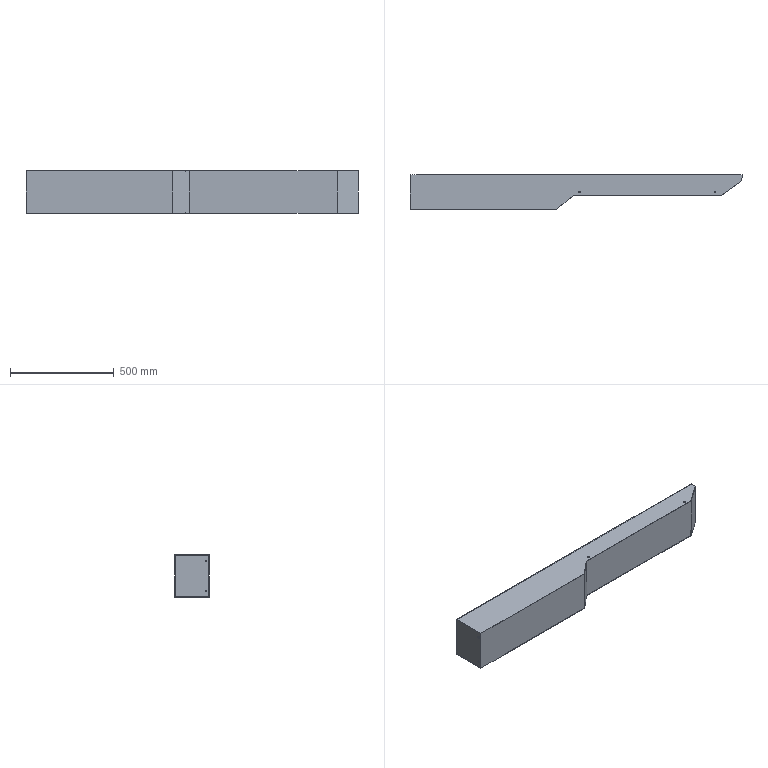Part | SolidWorks | features ICE 5, Extrusion 1, Shell 1 | 1 solid | 40 faces | box 1600 x 167 x 205 mm | volume 1759661 mm3 | plane 22 | cylinder 18 | commonest cylinder face diameters 9 x18
STEP:
#1=CARTESIAN_POINT('',(1474.53,-84.,-2.));
#2=VERTEX_POINT('',#1);
#3=CARTESIAN_POINT('',(1465.53,-84.,-2.));
#4=VERTEX_POINT('',#3);
#5=CARTESIAN_POINT('',(1470.03,-84.,-2.));
#6=DIRECTION('',(0.,0.,-1.));
#7=DIRECTION('',(-1.,0.,0.));
#8=AXIS2_PLACEMENT_3D('',#5,#6,#7);
#9=CIRCLE('',#8,4.5);
#10=EDGE_CURVE('',#2,#4,#9,.T.);
#11=ORIENTED_EDGE('',*,*,#10,.T.);
#12=CARTESIAN_POINT('',(1465.53,-84.,0.));
#13=VERTEX_POINT('',#12);
#14=CARTESIAN_POINT('',(1465.53,-84.,-110.));
#15=DIRECTION('',(0.,0.,1.));
#16=VECTOR('',#15,1000.);
#17=LINE('',#14,#16);
#18=EDGE_CURVE('',#4,#13,#17,.T.);
#19=ORIENTED_EDGE('',*,*,#18,.T.);
#20=CARTESIAN_POINT('',(1474.53,-84.,0.));
#21=VERTEX_POINT('',#20);
#22=CARTESIAN_POINT('',(1470.03,-84.,0.));
#23=DIRECTION('',(0.,0.,1.));
#24=DIRECTION('',(1.,0.,0.));
#25=AXIS2_PLACEMENT_3D('',#22,#23,#24);
#26=CIRCLE('',#25,4.5);
#27=EDGE_CURVE('',#13,#21,#26,.T.);
#28=ORIENTED_EDGE('',*,*,#27,.T.);
#29=CARTESIAN_POINT('',(1474.53,-84.,-110.));
#30=DIRECTION('',(0.,0.,1.));
#31=VECTOR('',#30,1000.);
#32=LINE('',#29,#31);
#33=EDGE_CURVE('',#2,#21,#32,.T.);
#34=ORIENTED_EDGE('',*,*,#33,.F.);
#35=EDGE_LOOP('',(#11,#19,#28,#34));
#36=FACE_OUTER_BOUND('',#35,.T.);
#37=CARTESIAN_POINT('',(1470.03,-84.,-110.));
#38=DIRECTION('',(0.,0.,1.));
#39=DIRECTION('',(1.,0.,0.));
#40=AXIS2_PLACEMENT_3D('',#37,#38,#39);
#41=CYLINDRICAL_SURFACE('',#40,4.5);
#42=ADVANCED_FACE('',(#36),#41,.F.);
#43=CARTESIAN_POINT('',(821.5,-84.,-2.));
#44=VERTEX_POINT('',#43);
#45=CARTESIAN_POINT('',(812.5,-84.,-2.));
#46=VERTEX_POINT('',#45);
#47=CARTESIAN_POINT('',(817.,-84.,-2.));
#48=DIRECTION('',(0.,0.,-1.));
#49=DIRECTION('',(-1.,0.,0.));
#50=AXIS2_PLACEMENT_3D('',#47,#48,#49);
#51=CIRCLE('',#50,4.5);
#52=EDGE_CURVE('',#44,#46,#51,.T.);
#53=ORIENTED_EDGE('',*,*,#52,.T.);
#54=CARTESIAN_POINT('',(812.5,-84.,0.));
#55=VERTEX_POINT('',#54);
#56=CARTESIAN_POINT('',(812.5,-84.,-110.));
#57=DIRECTION('',(0.,0.,1.));
#58=VECTOR('',#57,1000.);
#59=LINE('',#56,#58);
#60=EDGE_CURVE('',#46,#55,#59,.T.);
#61=ORIENTED_EDGE('',*,*,#60,.T.);
#62=CARTESIAN_POINT('',(821.5,-84.,0.));
#63=VERTEX_POINT('',#62);
#64=CARTESIAN_POINT('',(817.,-84.,0.));
#65=DIRECTION('',(0.,0.,1.));
#66=DIRECTION('',(1.,0.,0.));
#67=AXIS2_PLACEMENT_3D('',#64,#65,#66);
#68=CIRCLE('',#67,4.5);
#69=EDGE_CURVE('',#55,#63,#68,.T.);
#70=ORIENTED_EDGE('',*,*,#69,.T.);
#71=CARTESIAN_POINT('',(821.5,-84.,-110.));
#72=DIRECTION('',(0.,0.,1.));
#73=VECTOR('',#72,1000.);
#74=LINE('',#71,#73);
#75=EDGE_CURVE('',#44,#63,#74,.T.);
#76=ORIENTED_EDGE('',*,*,#75,.F.);
#77=EDGE_LOOP('',(#53,#61,#70,#76));
#78=FACE_OUTER_BOUND('',#77,.T.);
#79=CARTESIAN_POINT('',(817.,-84.,-110.));
#80=DIRECTION('',(0.,0.,1.));
#81=DIRECTION('',(1.,0.,0.));
#82=AXIS2_PLACEMENT_3D('',#79,#80,#81);
#83=CYLINDRICAL_SURFACE('',#82,4.5);
#84=ADVANCED_FACE('',(#78),#83,.F.);
#85=CARTESIAN_POINT('',(1588.5,-2.,-30.));
#86=VERTEX_POINT('',#85);
#87=CARTESIAN_POINT('',(1579.5,-2.,-30.));
#88=VERTEX_POINT('',#87);
#89=CARTESIAN_POINT('',(1584.,-2.,-30.));
#90=DIRECTION('',(0.,1.,0.));
#91=DIRECTION('',(-1.,0.,0.));
#92=AXIS2_PLACEMENT_3D('',#89,#90,#91);
#93=CIRCLE('',#92,4.5);
#94=EDGE_CURVE('',#86,#88,#93,.T.);
#95=ORIENTED_EDGE('',*,*,#94,.F.);
#96=CARTESIAN_POINT('',(1588.5,0.,-30.));
#97=VERTEX_POINT('',#96);
#98=CARTESIAN_POINT('',(1588.5,-16.,-30.));
#99=DIRECTION('',(0.,1.,0.));
#100=VECTOR('',#99,1000.);
#101=LINE('',#98,#100);
#102=EDGE_CURVE('',#86,#97,#101,.T.);
#103=ORIENTED_EDGE('',*,*,#102,.T.);
#104=CARTESIAN_POINT('',(1579.5,0.,-30.));
#105=VERTEX_POINT('',#104);
#106=CARTESIAN_POINT('',(1584.,0.,-30.));
#107=DIRECTION('',(0.,1.,0.));
#108=DIRECTION('',(-1.,0.,0.));
#109=AXIS2_PLACEMENT_3D('',#106,#107,#108);
#110=CIRCLE('',#109,4.5);
#111=EDGE_CURVE('',#97,#105,#110,.T.);
#112=ORIENTED_EDGE('',*,*,#111,.T.);
#113=CARTESIAN_POINT('',(1579.5,-16.,-30.));
#114=DIRECTION('',(0.,1.,0.));
#115=VECTOR('',#114,1000.);
#116=LINE('',#113,#115);
#117=EDGE_CURVE('',#88,#105,#116,.T.);
#118=ORIENTED_EDGE('',*,*,#117,.F.);
#119=EDGE_LOOP('',(#95,#103,#112,#118));
#120=FACE_OUTER_BOUND('',#119,.T.);
#121=CARTESIAN_POINT('',(1584.,-16.,-30.));
#122=DIRECTION('',(0.,1.,0.));
#123=DIRECTION('',(-1.,0.,0.));
#124=AXIS2_PLACEMENT_3D('',#121,#122,#123);
#125=CYLINDRICAL_SURFACE('',#124,4.5);
#126=ADVANCED_FACE('',(#120),#125,.F.);
#127=CARTESIAN_POINT('',(1588.5,-2.,-175.));
#128=VERTEX_POINT('',#127);
#129=CARTESIAN_POINT('',(1579.5,-2.,-175.));
#130=VERTEX_POINT('',#129);
#131=CARTESIAN_POINT('',(1584.,-2.,-175.));
#132=DIRECTION('',(0.,1.,0.));
#133=DIRECTION('',(-1.,0.,0.));
#134=AXIS2_PLACEMENT_3D('',#131,#132,#133);
#135=CIRCLE('',#134,4.5);
#136=EDGE_CURVE('',#128,#130,#135,.T.);
#137=ORIENTED_EDGE('',*,*,#136,.F.);
#138=CARTESIAN_POINT('',(1588.5,0.,-175.));
#139=VERTEX_POINT('',#138);
#140=CARTESIAN_POINT('',(1588.5,-16.,-175.));
#141=DIRECTION('',(0.,1.,0.));
#142=VECTOR('',#141,1000.);
#143=LINE('',#140,#142);
#144=EDGE_CURVE('',#128,#139,#143,.T.);
#145=ORIENTED_EDGE('',*,*,#144,.T.);
#146=CARTESIAN_POINT('',(1579.5,0.,-175.));
#147=VERTEX_POINT('',#146);
#148=CARTESIAN_POINT('',(1584.,0.,-175.));
#149=DIRECTION('',(0.,1.,0.));
#150=DIRECTION('',(-1.,0.,0.));
#151=AXIS2_PLACEMENT_3D('',#148,#149,#150);
#152=CIRCLE('',#151,4.5);
#153=EDGE_CURVE('',#139,#147,#152,.T.);
#154=ORIENTED_EDGE('',*,*,#153,.T.);
#155=CARTESIAN_POINT('',(1579.5,-16.,-175.));
#156=DIRECTION('',(0.,1.,0.));
#157=VECTOR('',#156,1000.);
#158=LINE('',#155,#157);
#159=EDGE_CURVE('',#130,#147,#158,.T.);
#160=ORIENTED_EDGE('',*,*,#159,.F.);
#161=EDGE_LOOP('',(#137,#145,#154,#160));
#162=FACE_OUTER_BOUND('',#161,.T.);
#163=CARTESIAN_POINT('',(1584.,-16.,-175.));
#164=DIRECTION('',(0.,1.,0.));
#165=DIRECTION('',(-1.,0.,0.));
#166=AXIS2_PLACEMENT_3D('',#163,#164,#165);
#167=CYLINDRICAL_SURFACE('',#166,4.5);
#168=ADVANCED_FACE('',(#162),#167,.F.);
#169=CARTESIAN_POINT('',(2.,-151.,-25.5));
#170=VERTEX_POINT('',#169);
#171=CARTESIAN_POINT('',(2.,-151.,-34.5));
#172=VERTEX_POINT('',#171);
#173=CARTESIAN_POINT('',(2.,-151.,-30.));
#174=DIRECTION('',(1.,0.,0.));
#175=DIRECTION('',(0.,0.,-1.));
#176=AXIS2_PLACEMENT_3D('',#173,#174,#175);
#177=CIRCLE('',#176,4.5);
#178=EDGE_CURVE('',#170,#172,#177,.T.);
#179=ORIENTED_EDGE('',*,*,#178,.T.);
#180=CARTESIAN_POINT('',(0.,-151.,-34.5));
#181=VERTEX_POINT('',#180);
#182=CARTESIAN_POINT('',(78.,-151.,-34.5));
#183=DIRECTION('',(-1.,0.,0.));
#184=VECTOR('',#183,1000.);
#185=LINE('',#182,#184);
#186=EDGE_CURVE('',#172,#181,#185,.T.);
#187=ORIENTED_EDGE('',*,*,#186,.T.);
#188=CARTESIAN_POINT('',(0.,-151.,-25.5));
#189=VERTEX_POINT('',#188);
#190=CARTESIAN_POINT('',(0.,-151.,-30.));
#191=DIRECTION('',(-1.,0.,0.));
#192=DIRECTION('',(0.,0.,1.));
#193=AXIS2_PLACEMENT_3D('',#190,#191,#192);
#194=CIRCLE('',#193,4.5);
#195=EDGE_CURVE('',#181,#189,#194,.T.);
#196=ORIENTED_EDGE('',*,*,#195,.T.);
#197=CARTESIAN_POINT('',(78.,-151.,-25.5));
#198=DIRECTION('',(-1.,0.,0.));
#199=VECTOR('',#198,1000.);
#200=LINE('',#197,#199);
#201=EDGE_CURVE('',#170,#189,#200,.T.);
#202=ORIENTED_EDGE('',*,*,#201,.F.);
#203=EDGE_LOOP('',(#179,#187,#196,#202));
#204=FACE_OUTER_BOUND('',#203,.T.);
#205=CARTESIAN_POINT('',(78.,-151.,-30.));
#206=DIRECTION('',(-1.,0.,0.));
#207=DIRECTION('',(0.,0.,1.));
#208=AXIS2_PLACEMENT_3D('',#205,#206,#207);
#209=CYLINDRICAL_SURFACE('',#208,4.5);
#210=ADVANCED_FACE('',(#204),#209,.F.);
#211=CARTESIAN_POINT('',(2.,-151.,-170.5));
#212=VERTEX_POINT('',#211);
#213=CARTESIAN_POINT('',(2.,-151.,-179.5));
#214=VERTEX_POINT('',#213);
#215=CARTESIAN_POINT('',(2.,-151.,-175.));
#216=DIRECTION('',(1.,0.,0.));
#217=DIRECTION('',(0.,0.,-1.));
#218=AXIS2_PLACEMENT_3D('',#215,#216,#217);
#219=CIRCLE('',#218,4.5);
#220=EDGE_CURVE('',#212,#214,#219,.T.);
#221=ORIENTED_EDGE('',*,*,#220,.T.);
#222=CARTESIAN_POINT('',(0.,-151.,-179.5));
#223=VERTEX_POINT('',#222);
#224=CARTESIAN_POINT('',(78.,-151.,-179.5));
#225=DIRECTION('',(-1.,0.,0.));
#226=VECTOR('',#225,1000.);
#227=LINE('',#224,#226);
#228=EDGE_CURVE('',#214,#223,#227,.T.);
#229=ORIENTED_EDGE('',*,*,#228,.T.);
#230=CARTESIAN_POINT('',(0.,-151.,-170.5));
#231=VERTEX_POINT('',#230);
#232=CARTESIAN_POINT('',(0.,-151.,-175.));
#233=DIRECTION('',(-1.,0.,0.));
#234=DIRECTION('',(0.,0.,1.));
#235=AXIS2_PLACEMENT_3D('',#232,#233,#234);
#236=CIRCLE('',#235,4.5);
#237=EDGE_CURVE('',#223,#231,#236,.T.);
#238=ORIENTED_EDGE('',*,*,#237,.T.);
#239=CARTESIAN_POINT('',(78.,-151.,-170.5));
#240=DIRECTION('',(-1.,0.,0.));
#241=VECTOR('',#240,1000.);
#242=LINE('',#239,#241);
#243=EDGE_CURVE('',#212,#231,#242,.T.);
#244=ORIENTED_EDGE('',*,*,#243,.F.);
#245=EDGE_LOOP('',(#221,#229,#238,#244));
#246=FACE_OUTER_BOUND('',#245,.T.);
#247=CARTESIAN_POINT('',(78.,-151.,-175.));
#248=DIRECTION('',(-1.,0.,0.));
#249=DIRECTION('',(0.,0.,1.));
#250=AXIS2_PLACEMENT_3D('',#247,#248,#249);
#251=CYLINDRICAL_SURFACE('',#250,4.5);
#252=ADVANCED_FACE('',(#246),#251,.F.);
#253=CARTESIAN_POINT('',(804.5,-14.,-203.));
#254=VERTEX_POINT('',#253);
#255=CARTESIAN_POINT('',(795.5,-14.,-203.));
#256=VERTEX_POINT('',#255);
#257=CARTESIAN_POINT('',(800.,-14.,-203.));
#258=DIRECTION('',(0.,0.,-1.));
#259=DIRECTION('',(-1.,0.,0.));
#260=AXIS2_PLACEMENT_3D('',#257,#258,#259);
#261=CIRCLE('',#260,4.5);
#262=EDGE_CURVE('',#254,#256,#261,.T.);
#263=ORIENTED_EDGE('',*,*,#262,.F.);
#264=CARTESIAN_POINT('',(804.5,-14.,-205.));
#265=VERTEX_POINT('',#264);
#266=CARTESIAN_POINT('',(804.5,-14.,-203.));
#267=DIRECTION('',(0.,0.,-1.));
#268=VECTOR('',#267,1000.);
#269=LINE('',#266,#268);
#270=EDGE_CURVE('',#254,#265,#269,.T.);
#271=ORIENTED_EDGE('',*,*,#270,.T.);
#272=CARTESIAN_POINT('',(795.5,-14.,-205.));
#273=VERTEX_POINT('',#272);
#274=CARTESIAN_POINT('',(800.,-14.,-205.));
#275=DIRECTION('',(0.,0.,-1.));
#276=DIRECTION('',(-1.,0.,0.));
#277=AXIS2_PLACEMENT_3D('',#274,#275,#276);
#278=CIRCLE('',#277,4.5);
#279=EDGE_CURVE('',#265,#273,#278,.T.);
#280=ORIENTED_EDGE('',*,*,#279,.T.);
#281=CARTESIAN_POINT('',(795.5,-14.,-203.));
#282=DIRECTION('',(0.,0.,-1.));
#283=VECTOR('',#282,1000.);
#284=LINE('',#281,#283);
#285=EDGE_CURVE('',#256,#273,#284,.T.);
#286=ORIENTED_EDGE('',*,*,#285,.F.);
#287=EDGE_LOOP('',(#263,#271,#280,#286));
#288=FACE_OUTER_BOUND('',#287,.T.);
#289=CARTESIAN_POINT('',(800.,-14.,-203.));
#290=DIRECTION('',(0.,0.,-1.));
#291=DIRECTION('',(-1.,0.,0.));
#292=AXIS2_PLACEMENT_3D('',#289,#290,#291);
#293=CYLINDRICAL_SURFACE('',#292,4.5);
#294=ADVANCED_FACE('',(#288),#293,.F.);
#295=CARTESIAN_POINT('',(34.5,-14.,-203.));
#296=VERTEX_POINT('',#295);
#297=CARTESIAN_POINT('',(25.5,-14.,-203.));
#298=VERTEX_POINT('',#297);
#299=CARTESIAN_POINT('',(30.,-14.,-203.));
#300=DIRECTION('',(0.,0.,-1.));
#301=DIRECTION('',(-1.,0.,0.));
#302=AXIS2_PLACEMENT_3D('',#299,#300,#301);
#303=CIRCLE('',#302,4.5);
#304=EDGE_CURVE('',#296,#298,#303,.T.);
#305=ORIENTED_EDGE('',*,*,#304,.F.);
#306=CARTESIAN_POINT('',(34.5,-14.,-205.));
#307=VERTEX_POINT('',#306);
#308=CARTESIAN_POINT('',(34.5,-14.,-203.));
#309=DIRECTION('',(0.,0.,-1.));
#310=VECTOR('',#309,1000.);
#311=LINE('',#308,#310);
#312=EDGE_CURVE('',#296,#307,#311,.T.);
#313=ORIENTED_EDGE('',*,*,#312,.T.);
#314=CARTESIAN_POINT('',(25.5,-14.,-205.));
#315=VERTEX_POINT('',#314);
#316=CARTESIAN_POINT('',(30.,-14.,-205.));
#317=DIRECTION('',(0.,0.,-1.));
#318=DIRECTION('',(-1.,0.,0.));
#319=AXIS2_PLACEMENT_3D('',#316,#317,#318);
#320=CIRCLE('',#319,4.5);
#321=EDGE_CURVE('',#307,#315,#320,.T.);
#322=ORIENTED_EDGE('',*,*,#321,.T.);
#323=CARTESIAN_POINT('',(25.5,-14.,-203.));
#324=DIRECTION('',(0.,0.,-1.));
#325=VECTOR('',#324,1000.);
#326=LINE('',#323,#325);
#327=EDGE_CURVE('',#298,#315,#326,.T.);
#328=ORIENTED_EDGE('',*,*,#327,.F.);
#329=EDGE_LOOP('',(#305,#313,#322,#328));
#330=FACE_OUTER_BOUND('',#329,.T.);
#331=CARTESIAN_POINT('',(30.,-14.,-203.));
#332=DIRECTION('',(0.,0.,-1.));
#333=DIRECTION('',(-1.,0.,0.));
#334=AXIS2_PLACEMENT_3D('',#331,#332,#333);
#335=CYLINDRICAL_SURFACE('',#334,4.5);
#336=ADVANCED_FACE('',(#330),#335,.F.);
#337=CARTESIAN_POINT('',(1574.5,-14.,-203.));
#338=VERTEX_POINT('',#337);
#339=CARTESIAN_POINT('',(1565.5,-14.,-203.));
#340=VERTEX_POINT('',#339);
#341=CARTESIAN_POINT('',(1570.,-14.,-203.));
#342=DIRECTION('',(0.,0.,-1.));
#343=DIRECTION('',(-1.,0.,0.));
#344=AXIS2_PLACEMENT_3D('',#341,#342,#343);
#345=CIRCLE('',#344,4.5);
#346=EDGE_CURVE('',#338,#340,#345,.T.);
#347=ORIENTED_EDGE('',*,*,#346,.F.);
#348=CARTESIAN_POINT('',(1574.5,-14.,-205.));
#349=VERTEX_POINT('',#348);
#350=CARTESIAN_POINT('',(1574.5,-14.,-203.));
#351=DIRECTION('',(0.,0.,-1.));
#352=VECTOR('',#351,1000.);
#353=LINE('',#350,#352);
#354=EDGE_CURVE('',#338,#349,#353,.T.);
#355=ORIENTED_EDGE('',*,*,#354,.T.);
#356=CARTESIAN_POINT('',(1565.5,-14.,-205.));
#357=VERTEX_POINT('',#356);
#358=CARTESIAN_POINT('',(1570.,-14.,-205.));
#359=DIRECTION('',(0.,0.,-1.));
#360=DIRECTION('',(-1.,0.,0.));
#361=AXIS2_PLACEMENT_3D('',#358,#359,#360);
#362=CIRCLE('',#361,4.5);
#363=EDGE_CURVE('',#349,#357,#362,.T.);
#364=ORIENTED_EDGE('',*,*,#363,.T.);
#365=CARTESIAN_POINT('',(1565.5,-14.,-203.));
#366=DIRECTION('',(0.,0.,-1.));
#367=VECTOR('',#366,1000.);
#368=LINE('',#365,#367);
#369=EDGE_CURVE('',#340,#357,#368,.T.);
#370=ORIENTED_EDGE('',*,*,#369,.F.);
#371=EDGE_LOOP('',(#347,#355,#364,#370));
#372=FACE_OUTER_BOUND('',#371,.T.);
#373=CARTESIAN_POINT('',(1570.,-14.,-203.));
#374=DIRECTION('',(0.,0.,-1.));
#375=DIRECTION('',(-1.,0.,0.));
#376=AXIS2_PLACEMENT_3D('',#373,#374,#375);
#377=CYLINDRICAL_SURFACE('',#376,4.5);
#378=ADVANCED_FACE('',(#372),#377,.F.);
#379=CARTESIAN_POINT('',(1584.,0.,-30.));
#380=DIRECTION('',(0.,1.,0.));
#381=DIRECTION('',(-1.,0.,0.));
#382=AXIS2_PLACEMENT_3D('',#379,#380,#381);
#383=CIRCLE('',#382,4.5);
#384=EDGE_CURVE('',#105,#97,#383,.T.);
#385=ORIENTED_EDGE('',*,*,#384,.F.);
#386=ORIENTED_EDGE('',*,*,#111,.F.);
#387=EDGE_LOOP('',(#385,#386));
#388=FACE_BOUND('',#387,.T.);
#389=CARTESIAN_POINT('',(1584.,0.,-175.));
#390=DIRECTION('',(0.,1.,0.));
#391=DIRECTION('',(-1.,0.,0.));
#392=AXIS2_PLACEMENT_3D('',#389,#390,#391);
#393=CIRCLE('',#392,4.5);
#394=EDGE_CURVE('',#147,#139,#393,.T.);
#395=ORIENTED_EDGE('',*,*,#394,.F.);
#396=ORIENTED_EDGE('',*,*,#153,.F.);
#397=EDGE_LOOP('',(#395,#396));
#398=FACE_BOUND('',#397,.T.);
#399=CARTESIAN_POINT('',(0.,0.,0.));
#400=VERTEX_POINT('',#399);
#401=CARTESIAN_POINT('',(1600.,0.,0.));
#402=VERTEX_POINT('',#401);
#403=CARTESIAN_POINT('',(0.,0.,0.));
#404=DIRECTION('',(1.,0.,0.));
#405=VECTOR('',#404,1000.);
#406=LINE('',#403,#405);
#407=EDGE_CURVE('',#400,#402,#406,.T.);
#408=ORIENTED_EDGE('',*,*,#407,.T.);
#409=CARTESIAN_POINT('',(1600.,0.,-205.));
#410=VERTEX_POINT('',#409);
#411=CARTESIAN_POINT('',(1600.,0.,-205.));
#412=DIRECTION('',(0.,0.,1.));
#413=VECTOR('',#412,1000.);
#414=LINE('',#411,#413);
#415=EDGE_CURVE('',#410,#402,#414,.T.);
#416=ORIENTED_EDGE('',*,*,#415,.F.);
#417=CARTESIAN_POINT('',(0.,0.,-205.));
#418=VERTEX_POINT('',#417);
#419=CARTESIAN_POINT('',(0.,0.,-205.));
#420=DIRECTION('',(1.,0.,0.));
#421=VECTOR('',#420,1000.);
#422=LINE('',#419,#421);
#423=EDGE_CURVE('',#418,#410,#422,.T.);
#424=ORIENTED_EDGE('',*,*,#423,.F.);
#425=CARTESIAN_POINT('',(0.,0.,-205.));
#426=DIRECTION('',(0.,0.,1.));
#427=VECTOR('',#426,1000.);
#428=LINE('',#425,#427);
#429=EDGE_CURVE('',#418,#400,#428,.T.);
#430=ORIENTED_EDGE('',*,*,#429,.T.);
#431=EDGE_LOOP('',(#408,#416,#424,#430));
#432=FACE_OUTER_BOUND('',#431,.T.);
#433=CARTESIAN_POINT('',(1570.,0.,-175.));
#434=VERTEX_POINT('',#433);
#435=CARTESIAN_POINT('',(30.,0.,-175.));
#436=VERTEX_POINT('',#435);
#437=CARTESIAN_POINT('',(30.,0.,-175.));
#438=DIRECTION('',(-1.,0.,0.));
#439=VECTOR('',#438,1000.);
#440=LINE('',#437,#439);
#441=EDGE_CURVE('',#434,#436,#440,.T.);
#442=ORIENTED_EDGE('',*,*,#441,.F.);
#443=CARTESIAN_POINT('',(1570.,0.,-30.));
#444=VERTEX_POINT('',#443);
#445=CARTESIAN_POINT('',(1570.,0.,-175.));
#446=DIRECTION('',(0.,0.,-1.));
#447=VECTOR('',#446,1000.);
#448=LINE('',#445,#447);
#449=EDGE_CURVE('',#444,#434,#448,.T.);
#450=ORIENTED_EDGE('',*,*,#449,.F.);
#451=CARTESIAN_POINT('',(30.,0.,-30.));
#452=VERTEX_POINT('',#451);
#453=CARTESIAN_POINT('',(30.,0.,-30.));
#454=DIRECTION('',(1.,0.,0.));
#455=VECTOR('',#454,1000.);
#456=LINE('',#453,#455);
#457=EDGE_CURVE('',#452,#444,#456,.T.);
#458=ORIENTED_EDGE('',*,*,#457,.F.);
#459=CARTESIAN_POINT('',(30.,0.,-175.));
#460=DIRECTION('',(0.,0.,1.));
#461=VECTOR('',#460,1000.);
#462=LINE('',#459,#461);
#463=EDGE_CURVE('',#436,#452,#462,.T.);
#464=ORIENTED_EDGE('',*,*,#463,.F.);
#465=EDGE_LOOP('',(#442,#450,#458,#464));
#466=FACE_BOUND('',#465,.T.);
#467=CARTESIAN_POINT('',(0.,0.,-205.));
#468=DIRECTION('',(0.,-1.,0.));
#469=DIRECTION('',(1.,0.,0.));
#470=AXIS2_PLACEMENT_3D('',#467,#468,#469);
#471=PLANE('',#470);
#472=ADVANCED_FACE('',(#388,#398,#432,#466),#471,.F.);
#473=CARTESIAN_POINT('',(1500.03,-100.,0.));
#474=VERTEX_POINT('',#473);
#475=CARTESIAN_POINT('',(787.,-100.,0.));
#476=VERTEX_POINT('',#475);
#477=CARTESIAN_POINT('',(1500.03,-100.,0.));
#478=DIRECTION('',(-1.,0.,0.));
#479=VECTOR('',#478,1000.);
#480=LINE('',#477,#479);
#481=EDGE_CURVE('',#474,#476,#480,.T.);
#482=ORIENTED_EDGE('',*,*,#481,.T.);
#483=CARTESIAN_POINT('',(787.,-100.,-205.));
#484=VERTEX_POINT('',#483);
#485=CARTESIAN_POINT('',(787.,-100.,-205.));
#486=DIRECTION('',(0.,0.,1.));
#487=VECTOR('',#486,1000.);
#488=LINE('',#485,#487);
#489=EDGE_CURVE('',#484,#476,#488,.T.);
#490=ORIENTED_EDGE('',*,*,#489,.F.);
#491=CARTESIAN_POINT('',(1500.03,-100.,-205.));
#492=VERTEX_POINT('',#491);
#493=CARTESIAN_POINT('',(1500.03,-100.,-205.));
#494=DIRECTION('',(-1.,0.,0.));
#495=VECTOR('',#494,1000.);
#496=LINE('',#493,#495);
#497=EDGE_CURVE('',#492,#484,#496,.T.);
#498=ORIENTED_EDGE('',*,*,#497,.F.);
#499=CARTESIAN_POINT('',(1500.03,-100.,-205.));
#500=DIRECTION('',(0.,0.,1.));
#501=VECTOR('',#500,1000.);
#502=LINE('',#499,#501);
#503=EDGE_CURVE('',#492,#474,#502,.T.);
#504=ORIENTED_EDGE('',*,*,#503,.T.);
#505=EDGE_LOOP('',(#482,#490,#498,#504));
#506=FACE_OUTER_BOUND('',#505,.T.);
#507=CARTESIAN_POINT('',(1500.03,-100.,-205.));
#508=DIRECTION('',(0.,1.,0.));
#509=DIRECTION('',(-1.,0.,0.));
#510=AXIS2_PLACEMENT_3D('',#507,#508,#509);
#511=PLANE('',#510);
#512=ADVANCED_FACE('',(#506),#511,.F.);
#513=CARTESIAN_POINT('',(707.153,-167.,0.));
#514=VERTEX_POINT('',#513);
#515=CARTESIAN_POINT('',(787.,-100.,0.));
#516=DIRECTION('',(-0.766,-0.6428,0.));
#517=VECTOR('',#516,1000.);
#518=LINE('',#515,#517);
#519=EDGE_CURVE('',#476,#514,#518,.T.);
#520=ORIENTED_EDGE('',*,*,#519,.T.);
#521=CARTESIAN_POINT('',(707.153,-167.,-205.));
#522=VERTEX_POINT('',#521);
#523=CARTESIAN_POINT('',(707.153,-167.,-205.));
#524=DIRECTION('',(0.,0.,1.));
#525=VECTOR('',#524,1000.);
#526=LINE('',#523,#525);
#527=EDGE_CURVE('',#522,#514,#526,.T.);
#528=ORIENTED_EDGE('',*,*,#527,.F.);
#529=CARTESIAN_POINT('',(787.,-100.,-205.));
#530=DIRECTION('',(-0.766,-0.6428,0.));
#531=VECTOR('',#530,1000.);
#532=LINE('',#529,#531);
#533=EDGE_CURVE('',#484,#522,#532,.T.);
#534=ORIENTED_EDGE('',*,*,#533,.F.);
#535=ORIENTED_EDGE('',*,*,#489,.T.);
#536=EDGE_LOOP('',(#520,#528,#534,#535));
#537=FACE_OUTER_BOUND('',#536,.T.);
#538=CARTESIAN_POINT('',(787.,-100.,-205.));
#539=DIRECTION('',(-0.6428,0.766,0.));
#540=DIRECTION('',(-0.766,-0.6428,0.));
#541=AXIS2_PLACEMENT_3D('',#538,#539,#540);
#542=PLANE('',#541);
#543=ADVANCED_FACE('',(#537),#542,.F.);
#544=CARTESIAN_POINT('',(0.,-167.,0.));
#545=VERTEX_POINT('',#544);
#546=CARTESIAN_POINT('',(707.153,-167.,0.));
#547=DIRECTION('',(-1.,0.,0.));
#548=VECTOR('',#547,1000.);
#549=LINE('',#546,#548);
#550=EDGE_CURVE('',#514,#545,#549,.T.);
#551=ORIENTED_EDGE('',*,*,#550,.T.);
#552=CARTESIAN_POINT('',(0.,-167.,-205.));
#553=VERTEX_POINT('',#552);
#554=CARTESIAN_POINT('',(0.,-167.,-205.));
#555=DIRECTION('',(0.,0.,1.));
#556=VECTOR('',#555,1000.);
#557=LINE('',#554,#556);
#558=EDGE_CURVE('',#553,#545,#557,.T.);
#559=ORIENTED_EDGE('',*,*,#558,.F.);
#560=CARTESIAN_POINT('',(707.153,-167.,-205.));
#561=DIRECTION('',(-1.,0.,0.));
#562=VECTOR('',#561,1000.);
#563=LINE('',#560,#562);
#564=EDGE_CURVE('',#522,#553,#563,.T.);
#565=ORIENTED_EDGE('',*,*,#564,.F.);
#566=ORIENTED_EDGE('',*,*,#527,.T.);
#567=EDGE_LOOP('',(#551,#559,#565,#566));
#568=FACE_OUTER_BOUND('',#567,.T.);
#569=CARTESIAN_POINT('',(707.153,-167.,-205.));
#570=DIRECTION('',(0.,1.,0.));
#571=DIRECTION('',(-1.,0.,0.));
#572=AXIS2_PLACEMENT_3D('',#569,#570,#571);
#573=PLANE('',#572);
#574=ADVANCED_FACE('',(#568),#573,.F.);
#575=CARTESIAN_POINT('',(0.,-151.,-30.));
#576=DIRECTION('',(-1.,0.,0.));
#577=DIRECTION('',(0.,0.,1.));
#578=AXIS2_PLACEMENT_3D('',#575,#576,#577);
#579=CIRCLE('',#578,4.5);
#580=EDGE_CURVE('',#189,#181,#579,.T.);
#581=ORIENTED_EDGE('',*,*,#580,.F.);
#582=ORIENTED_EDGE('',*,*,#195,.F.);
#583=EDGE_LOOP('',(#581,#582));
#584=FACE_BOUND('',#583,.T.);
#585=CARTESIAN_POINT('',(0.,-151.,-175.));
#586=DIRECTION('',(-1.,0.,0.));
#587=DIRECTION('',(0.,0.,1.));
#588=AXIS2_PLACEMENT_3D('',#585,#586,#587);
#589=CIRCLE('',#588,4.5);
#590=EDGE_CURVE('',#231,#223,#589,.T.);
#591=ORIENTED_EDGE('',*,*,#590,.F.);
#592=ORIENTED_EDGE('',*,*,#237,.F.);
#593=EDGE_LOOP('',(#591,#592));
#594=FACE_BOUND('',#593,.T.);
#595=ORIENTED_EDGE('',*,*,#429,.F.);
#596=CARTESIAN_POINT('',(0.,-167.,-205.));
#597=DIRECTION('',(0.,1.,0.));
#598=VECTOR('',#597,1000.);
#599=LINE('',#596,#598);
#600=EDGE_CURVE('',#553,#418,#599,.T.);
#601=ORIENTED_EDGE('',*,*,#600,.F.);
#602=ORIENTED_EDGE('',*,*,#558,.T.);
#603=CARTESIAN_POINT('',(0.,-167.,0.));
#604=DIRECTION('',(0.,1.,0.));
#605=VECTOR('',#604,1000.);
#606=LINE('',#603,#605);
#607=EDGE_CURVE('',#545,#400,#606,.T.);
#608=ORIENTED_EDGE('',*,*,#607,.T.);
#609=EDGE_LOOP('',(#595,#601,#602,#608));
#610=FACE_OUTER_BOUND('',#609,.T.);
#611=CARTESIAN_POINT('',(0.,-167.,-205.));
#612=DIRECTION('',(1.,0.,0.));
#613=DIRECTION('',(0.,0.,-1.));
#614=AXIS2_PLACEMENT_3D('',#611,#612,#613);
#615=PLANE('',#614);
#616=ADVANCED_FACE('',(#584,#594,#610),#615,.F.);
#617=CARTESIAN_POINT('',(1600.,-30.,0.));
#618=VERTEX_POINT('',#617);
#619=CARTESIAN_POINT('',(1600.,0.,0.));
#620=DIRECTION('',(0.,-1.,0.));
#621=VECTOR('',#620,1000.);
#622=LINE('',#619,#621);
#623=EDGE_CURVE('',#402,#618,#622,.T.);
#624=ORIENTED_EDGE('',*,*,#623,.T.);
#625=CARTESIAN_POINT('',(1600.,-30.,-205.));
#626=VERTEX_POINT('',#625);
#627=CARTESIAN_POINT('',(1600.,-30.,-205.));
#628=DIRECTION('',(0.,0.,1.));
#629=VECTOR('',#628,1000.);
#630=LINE('',#627,#629);
#631=EDGE_CURVE('',#626,#618,#630,.T.);
#632=ORIENTED_EDGE('',*,*,#631,.F.);
#633=CARTESIAN_POINT('',(1600.,0.,-205.));
#634=DIRECTION('',(0.,-1.,0.));
#635=VECTOR('',#634,1000.);
#636=LINE('',#633,#635);
#637=EDGE_CURVE('',#410,#626,#636,.T.);
#638=ORIENTED_EDGE('',*,*,#637,.F.);
#639=ORIENTED_EDGE('',*,*,#415,.T.);
#640=EDGE_LOOP('',(#624,#632,#638,#639));
#641=FACE_OUTER_BOUND('',#640,.T.);
#642=CARTESIAN_POINT('',(1600.,0.,-205.));
#643=DIRECTION('',(-1.,0.,0.));
#644=DIRECTION('',(0.,-1.,0.));
#645=AXIS2_PLACEMENT_3D('',#642,#643,#644);
#646=PLANE('',#645);
#647=ADVANCED_FACE('',(#641),#646,.F.);
#648=CARTESIAN_POINT('',(1600.,-30.,0.));
#649=DIRECTION('',(-0.8192,-0.5736,0.));
#650=VECTOR('',#649,1000.);
#651=LINE('',#648,#650);
#652=EDGE_CURVE('',#618,#474,#651,.T.);
#653=ORIENTED_EDGE('',*,*,#652,.T.);
#654=ORIENTED_EDGE('',*,*,#503,.F.);
#655=CARTESIAN_POINT('',(1600.,-30.,-205.));
#656=DIRECTION('',(-0.8192,-0.5736,0.));
#657=VECTOR('',#656,1000.);
#658=LINE('',#655,#657);
#659=EDGE_CURVE('',#626,#492,#658,.T.);
#660=ORIENTED_EDGE('',*,*,#659,.F.);
#661=ORIENTED_EDGE('',*,*,#631,.T.);
#662=EDGE_LOOP('',(#653,#654,#660,#661));
#663=FACE_OUTER_BOUND('',#662,.T.);
#664=CARTESIAN_POINT('',(1600.,-30.,-205.));
#665=DIRECTION('',(-0.5736,0.8192,0.));
#666=DIRECTION('',(-0.8192,-0.5736,0.));
#667=AXIS2_PLACEMENT_3D('',#664,#665,#666);
#668=PLANE('',#667);
#669=ADVANCED_FACE('',(#663),#668,.F.);
#670=CARTESIAN_POINT('',(800.,-14.,-205.));
#671=DIRECTION('',(0.,0.,-1.));
#672=DIRECTION('',(-1.,0.,0.));
#673=AXIS2_PLACEMENT_3D('',#670,#671,#672);
#674=CIRCLE('',#673,4.5);
#675=EDGE_CURVE('',#273,#265,#674,.T.);
#676=ORIENTED_EDGE('',*,*,#675,.F.);
#677=ORIENTED_EDGE('',*,*,#279,.F.);
#678=EDGE_LOOP('',(#676,#677));
#679=FACE_BOUND('',#678,.T.);
#680=CARTESIAN_POINT('',(30.,-14.,-205.));
#681=DIRECTION('',(0.,0.,-1.));
#682=DIRECTION('',(-1.,0.,0.));
#683=AXIS2_PLACEMENT_3D('',#680,#681,#682);
#684=CIRCLE('',#683,4.5);
#685=EDGE_CURVE('',#315,#307,#684,.T.);
#686=ORIENTED_EDGE('',*,*,#685,.F.);
#687=ORIENTED_EDGE('',*,*,#321,.F.);
#688=EDGE_LOOP('',(#686,#687));
#689=FACE_BOUND('',#688,.T.);
#690=CARTESIAN_POINT('',(1570.,-14.,-205.));
#691=DIRECTION('',(0.,0.,-1.));
#692=DIRECTION('',(-1.,0.,0.));
#693=AXIS2_PLACEMENT_3D('',#690,#691,#692);
#694=CIRCLE('',#693,4.5);
#695=EDGE_CURVE('',#357,#349,#694,.T.);
#696=ORIENTED_EDGE('',*,*,#695,.F.);
#697=ORIENTED_EDGE('',*,*,#363,.F.);
#698=EDGE_LOOP('',(#696,#697));
#699=FACE_BOUND('',#698,.T.);
#700=ORIENTED_EDGE('',*,*,#637,.T.);
#701=ORIENTED_EDGE('',*,*,#659,.T.);
#702=ORIENTED_EDGE('',*,*,#497,.T.);
#703=ORIENTED_EDGE('',*,*,#533,.T.);
#704=ORIENTED_EDGE('',*,*,#564,.T.);
#705=ORIENTED_EDGE('',*,*,#600,.T.);
#706=ORIENTED_EDGE('',*,*,#423,.T.);
#707=EDGE_LOOP('',(#700,#701,#702,#703,#704,#705,#706));
#708=FACE_OUTER_BOUND('',#707,.T.);
#709=CARTESIAN_POINT('',(0.,-100.,-205.));
#710=DIRECTION('',(0.,0.,-1.));
#711=DIRECTION('',(-1.,0.,0.));
#712=AXIS2_PLACEMENT_3D('',#709,#710,#711);
#713=PLANE('',#712);
#714=ADVANCED_FACE('',(#679,#689,#699,#708),#713,.T.);
#715=CARTESIAN_POINT('',(1470.03,-84.,0.));
#716=DIRECTION('',(0.,0.,1.));
#717=DIRECTION('',(1.,0.,0.));
#718=AXIS2_PLACEMENT_3D('',#715,#716,#717);
#719=CIRCLE('',#718,4.5);
#720=EDGE_CURVE('',#21,#13,#719,.T.);
#721=ORIENTED_EDGE('',*,*,#720,.F.);
#722=ORIENTED_EDGE('',*,*,#27,.F.);
#723=EDGE_LOOP('',(#721,#722));
#724=FACE_BOUND('',#723,.T.);
#725=CARTESIAN_POINT('',(817.,-84.,0.));
#726=DIRECTION('',(0.,0.,1.));
#727=DIRECTION('',(1.,0.,0.));
#728=AXIS2_PLACEMENT_3D('',#725,#726,#727);
#729=CIRCLE('',#728,4.5);
#730=EDGE_CURVE('',#63,#55,#729,.T.);
#731=ORIENTED_EDGE('',*,*,#730,.F.);
#732=ORIENTED_EDGE('',*,*,#69,.F.);
#733=EDGE_LOOP('',(#731,#732));
#734=FACE_BOUND('',#733,.T.);
#735=ORIENTED_EDGE('',*,*,#407,.F.);
#736=ORIENTED_EDGE('',*,*,#607,.F.);
#737=ORIENTED_EDGE('',*,*,#550,.F.);
#738=ORIENTED_EDGE('',*,*,#519,.F.);
#739=ORIENTED_EDGE('',*,*,#481,.F.);
#740=ORIENTED_EDGE('',*,*,#652,.F.);
#741=ORIENTED_EDGE('',*,*,#623,.F.);
#742=EDGE_LOOP('',(#735,#736,#737,#738,#739,#740,#741));
#743=FACE_OUTER_BOUND('',#742,.T.);
#744=CARTESIAN_POINT('',(0.,-100.,0.));
#745=DIRECTION('',(0.,0.,-1.));
#746=DIRECTION('',(-1.,0.,0.));
#747=AXIS2_PLACEMENT_3D('',#744,#745,#746);
#748=PLANE('',#747);
#749=ADVANCED_FACE('',(#724,#734,#743),#748,.F.);
#750=CARTESIAN_POINT('',(1584.,-2.,-30.));
#751=DIRECTION('',(0.,1.,0.));
#752=DIRECTION('',(-1.,0.,0.));
#753=AXIS2_PLACEMENT_3D('',#750,#751,#752);
#754=CIRCLE('',#753,4.5);
#755=EDGE_CURVE('',#88,#86,#754,.T.);
#756=ORIENTED_EDGE('',*,*,#755,.T.);
#757=ORIENTED_EDGE('',*,*,#94,.T.);
#758=EDGE_LOOP('',(#756,#757));
#759=FACE_BOUND('',#758,.T.);
#760=CARTESIAN_POINT('',(1584.,-2.,-175.));
#761=DIRECTION('',(0.,1.,0.));
#762=DIRECTION('',(-1.,0.,0.));
#763=AXIS2_PLACEMENT_3D('',#760,#761,#762);
#764=CIRCLE('',#763,4.5);
#765=EDGE_CURVE('',#130,#128,#764,.T.);
#766=ORIENTED_EDGE('',*,*,#765,.T.);
#767=ORIENTED_EDGE('',*,*,#136,.T.);
#768=EDGE_LOOP('',(#766,#767));
#769=FACE_BOUND('',#768,.T.);
#770=CARTESIAN_POINT('',(1570.,-2.,-30.));
#771=VERTEX_POINT('',#770);
#772=CARTESIAN_POINT('',(1570.,-2.,-175.));
#773=VERTEX_POINT('',#772);
#774=CARTESIAN_POINT('',(1570.,-2.,-175.));
#775=DIRECTION('',(0.,0.,-1.));
#776=VECTOR('',#775,1000.);
#777=LINE('',#774,#776);
#778=EDGE_CURVE('',#771,#773,#777,.T.);
#779=ORIENTED_EDGE('',*,*,#778,.T.);
#780=CARTESIAN_POINT('',(30.,-2.,-175.));
#781=VERTEX_POINT('',#780);
#782=CARTESIAN_POINT('',(30.,-2.,-175.));
#783=DIRECTION('',(-1.,0.,0.));
#784=VECTOR('',#783,1000.);
#785=LINE('',#782,#784);
#786=EDGE_CURVE('',#773,#781,#785,.T.);
#787=ORIENTED_EDGE('',*,*,#786,.T.);
#788=CARTESIAN_POINT('',(30.,-2.,-30.));
#789=VERTEX_POINT('',#788);
#790=CARTESIAN_POINT('',(30.,-2.,-175.));
#791=DIRECTION('',(0.,0.,1.));
#792=VECTOR('',#791,1000.);
#793=LINE('',#790,#792);
#794=EDGE_CURVE('',#781,#789,#793,.T.);
#795=ORIENTED_EDGE('',*,*,#794,.T.);
#796=CARTESIAN_POINT('',(30.,-2.,-30.));
#797=DIRECTION('',(1.,0.,0.));
#798=VECTOR('',#797,1000.);
#799=LINE('',#796,#798);
#800=EDGE_CURVE('',#789,#771,#799,.T.);
#801=ORIENTED_EDGE('',*,*,#800,.T.);
#802=EDGE_LOOP('',(#779,#787,#795,#801));
#803=FACE_BOUND('',#802,.T.);
#804=CARTESIAN_POINT('',(2.,-2.,-203.));
#805=VERTEX_POINT('',#804);
#806=CARTESIAN_POINT('',(2.,-2.,-2.));
#807=VERTEX_POINT('',#806);
#808=CARTESIAN_POINT('',(2.,-2.,-205.));
#809=DIRECTION('',(0.,0.,1.));
#810=VECTOR('',#809,1000.);
#811=LINE('',#808,#810);
#812=EDGE_CURVE('',#805,#807,#811,.T.);
#813=ORIENTED_EDGE('',*,*,#812,.F.);
#814=CARTESIAN_POINT('',(1598.,-2.,-203.));
#815=VERTEX_POINT('',#814);
#816=CARTESIAN_POINT('',(0.,-2.,-203.));
#817=DIRECTION('',(1.,0.,0.));
#818=VECTOR('',#817,1000.);
#819=LINE('',#816,#818);
#820=EDGE_CURVE('',#805,#815,#819,.T.);
#821=ORIENTED_EDGE('',*,*,#820,.T.);
#822=CARTESIAN_POINT('',(1598.,-2.,-2.));
#823=VERTEX_POINT('',#822);
#824=CARTESIAN_POINT('',(1598.,-2.,-205.));
#825=DIRECTION('',(0.,0.,-1.));
#826=VECTOR('',#825,1000.);
#827=LINE('',#824,#826);
#828=EDGE_CURVE('',#823,#815,#827,.T.);
#829=ORIENTED_EDGE('',*,*,#828,.F.);
#830=CARTESIAN_POINT('',(0.,-2.,-2.));
#831=DIRECTION('',(1.,0.,0.));
#832=VECTOR('',#831,1000.);
#833=LINE('',#830,#832);
#834=EDGE_CURVE('',#807,#823,#833,.T.);
#835=ORIENTED_EDGE('',*,*,#834,.F.);
#836=EDGE_LOOP('',(#813,#821,#829,#835));
#837=FACE_OUTER_BOUND('',#836,.T.);
#838=CARTESIAN_POINT('',(0.,-2.,0.));
#839=DIRECTION('',(0.,1.,0.));
#840=DIRECTION('',(-1.,0.,0.));
#841=AXIS2_PLACEMENT_3D('',#838,#839,#840);
#842=PLANE('',#841);
#843=ADVANCED_FACE('',(#759,#769,#803,#837),#842,.F.);
#844=ORIENTED_EDGE('',*,*,#441,.T.);
#845=CARTESIAN_POINT('',(30.,-2.,-175.));
#846=DIRECTION('',(0.,1.,0.));
#847=VECTOR('',#846,1000.);
#848=LINE('',#845,#847);
#849=EDGE_CURVE('',#781,#436,#848,.T.);
#850=ORIENTED_EDGE('',*,*,#849,.F.);
#851=ORIENTED_EDGE('',*,*,#786,.F.);
#852=CARTESIAN_POINT('',(1570.,-2.,-175.));
#853=DIRECTION('',(0.,1.,0.));
#854=VECTOR('',#853,1000.);
#855=LINE('',#852,#854);
#856=EDGE_CURVE('',#773,#434,#855,.T.);
#857=ORIENTED_EDGE('',*,*,#856,.T.);
#858=EDGE_LOOP('',(#844,#850,#851,#857));
#859=FACE_OUTER_BOUND('',#858,.T.);
#860=CARTESIAN_POINT('',(30.,-2.,-175.));
#861=DIRECTION('',(0.,0.,-1.));
#862=DIRECTION('',(0.,1.,0.));
#863=AXIS2_PLACEMENT_3D('',#860,#861,#862);
#864=PLANE('',#863);
#865=ADVANCED_FACE('',(#859),#864,.F.);
#866=ORIENTED_EDGE('',*,*,#449,.T.);
#867=ORIENTED_EDGE('',*,*,#856,.F.);
#868=ORIENTED_EDGE('',*,*,#778,.F.);
#869=CARTESIAN_POINT('',(1570.,-2.,-30.));
#870=DIRECTION('',(0.,1.,0.));
#871=VECTOR('',#870,1000.);
#872=LINE('',#869,#871);
#873=EDGE_CURVE('',#771,#444,#872,.T.);
#874=ORIENTED_EDGE('',*,*,#873,.T.);
#875=EDGE_LOOP('',(#866,#867,#868,#874));
#876=FACE_OUTER_BOUND('',#875,.T.);
#877=CARTESIAN_POINT('',(1570.,-2.,-175.));
#878=DIRECTION('',(1.,0.,0.));
#879=DIRECTION('',(0.,1.,0.));
#880=AXIS2_PLACEMENT_3D('',#877,#878,#879);
#881=PLANE('',#880);
#882=ADVANCED_FACE('',(#876),#881,.F.);
#883=ORIENTED_EDGE('',*,*,#457,.T.);
#884=ORIENTED_EDGE('',*,*,#873,.F.);
#885=ORIENTED_EDGE('',*,*,#800,.F.);
#886=CARTESIAN_POINT('',(30.,-2.,-30.));
#887=DIRECTION('',(0.,1.,0.));
#888=VECTOR('',#887,1000.);
#889=LINE('',#886,#888);
#890=EDGE_CURVE('',#789,#452,#889,.T.);
#891=ORIENTED_EDGE('',*,*,#890,.T.);
#892=EDGE_LOOP('',(#883,#884,#885,#891));
#893=FACE_OUTER_BOUND('',#892,.T.);
#894=CARTESIAN_POINT('',(30.,-2.,-30.));
#895=DIRECTION('',(0.,0.,1.));
#896=DIRECTION('',(1.,0.,0.));
#897=AXIS2_PLACEMENT_3D('',#894,#895,#896);
#898=PLANE('',#897);
#899=ADVANCED_FACE('',(#893),#898,.F.);
#900=ORIENTED_EDGE('',*,*,#463,.T.);
#901=ORIENTED_EDGE('',*,*,#890,.F.);
#902=ORIENTED_EDGE('',*,*,#794,.F.);
#903=ORIENTED_EDGE('',*,*,#849,.T.);
#904=EDGE_LOOP('',(#900,#901,#902,#903));
#905=FACE_OUTER_BOUND('',#904,.T.);
#906=CARTESIAN_POINT('',(30.,-2.,-175.));
#907=DIRECTION('',(-1.,0.,0.));
#908=DIRECTION('',(0.,-1.,0.));
#909=AXIS2_PLACEMENT_3D('',#906,#907,#908);
#910=PLANE('',#909);
#911=ADVANCED_FACE('',(#905),#910,.F.);
#912=CARTESIAN_POINT('',(706.425,-165.,-2.));
#913=VERTEX_POINT('',#912);
#914=CARTESIAN_POINT('',(2.,-165.,-2.));
#915=VERTEX_POINT('',#914);
#916=CARTESIAN_POINT('',(707.153,-165.,-2.));
#917=DIRECTION('',(-1.,0.,0.));
#918=VECTOR('',#917,1000.);
#919=LINE('',#916,#918);
#920=EDGE_CURVE('',#913,#915,#919,.T.);
#921=ORIENTED_EDGE('',*,*,#920,.F.);
#922=CARTESIAN_POINT('',(706.425,-165.,-203.));
#923=VERTEX_POINT('',#922);
#924=CARTESIAN_POINT('',(706.425,-165.,-205.));
#925=DIRECTION('',(0.,0.,1.));
#926=VECTOR('',#925,1000.);
#927=LINE('',#924,#926);
#928=EDGE_CURVE('',#923,#913,#927,.T.);
#929=ORIENTED_EDGE('',*,*,#928,.F.);
#930=CARTESIAN_POINT('',(2.,-165.,-203.));
#931=VERTEX_POINT('',#930);
#932=CARTESIAN_POINT('',(707.153,-165.,-203.));
#933=DIRECTION('',(-1.,0.,0.));
#934=VECTOR('',#933,1000.);
#935=LINE('',#932,#934);
#936=EDGE_CURVE('',#923,#931,#935,.T.);
#937=ORIENTED_EDGE('',*,*,#936,.T.);
#938=CARTESIAN_POINT('',(2.,-165.,-205.));
#939=DIRECTION('',(0.,0.,1.));
#940=VECTOR('',#939,1000.);
#941=LINE('',#938,#940);
#942=EDGE_CURVE('',#931,#915,#941,.T.);
#943=ORIENTED_EDGE('',*,*,#942,.T.);
#944=EDGE_LOOP('',(#921,#929,#937,#943));
#945=FACE_OUTER_BOUND('',#944,.T.);
#946=CARTESIAN_POINT('',(707.153,-165.,-205.));
#947=DIRECTION('',(0.,1.,0.));
#948=DIRECTION('',(-1.,0.,0.));
#949=AXIS2_PLACEMENT_3D('',#946,#947,#948);
#950=PLANE('',#949);
#951=ADVANCED_FACE('',(#945),#950,.T.);
#952=CARTESIAN_POINT('',(786.272,-98.,-2.));
#953=VERTEX_POINT('',#952);
#954=CARTESIAN_POINT('',(785.714,-98.468,-2.));
#955=DIRECTION('',(-0.766,-0.6428,0.));
#956=VECTOR('',#955,1000.);
#957=LINE('',#954,#956);
#958=EDGE_CURVE('',#953,#913,#957,.T.);
#959=ORIENTED_EDGE('',*,*,#958,.F.);
#960=CARTESIAN_POINT('',(786.272,-98.,-203.));
#961=VERTEX_POINT('',#960);
#962=CARTESIAN_POINT('',(786.272,-98.,-205.));
#963=DIRECTION('',(0.,0.,1.));
#964=VECTOR('',#963,1000.);
#965=LINE('',#962,#964);
#966=EDGE_CURVE('',#961,#953,#965,.T.);
#967=ORIENTED_EDGE('',*,*,#966,.F.);
#968=CARTESIAN_POINT('',(785.714,-98.468,-203.));
#969=DIRECTION('',(-0.766,-0.6428,0.));
#970=VECTOR('',#969,1000.);
#971=LINE('',#968,#970);
#972=EDGE_CURVE('',#961,#923,#971,.T.);
#973=ORIENTED_EDGE('',*,*,#972,.T.);
#974=ORIENTED_EDGE('',*,*,#928,.T.);
#975=EDGE_LOOP('',(#959,#967,#973,#974));
#976=FACE_OUTER_BOUND('',#975,.T.);
#977=CARTESIAN_POINT('',(785.714,-98.468,-205.));
#978=DIRECTION('',(-0.6428,0.766,0.));
#979=DIRECTION('',(-0.766,-0.6428,0.));
#980=AXIS2_PLACEMENT_3D('',#977,#978,#979);
#981=PLANE('',#980);
#982=ADVANCED_FACE('',(#976),#981,.T.);
#983=CARTESIAN_POINT('',(1499.399,-98.,-2.));
#984=VERTEX_POINT('',#983);
#985=CARTESIAN_POINT('',(1500.03,-98.,-2.));
#986=DIRECTION('',(-1.,0.,0.));
#987=VECTOR('',#986,1000.);
#988=LINE('',#985,#987);
#989=EDGE_CURVE('',#984,#953,#988,.T.);
#990=ORIENTED_EDGE('',*,*,#989,.F.);
#991=CARTESIAN_POINT('',(1499.399,-98.,-203.));
#992=VERTEX_POINT('',#991);
#993=CARTESIAN_POINT('',(1499.399,-98.,-205.));
#994=DIRECTION('',(0.,0.,1.));
#995=VECTOR('',#994,1000.);
#996=LINE('',#993,#995);
#997=EDGE_CURVE('',#992,#984,#996,.T.);
#998=ORIENTED_EDGE('',*,*,#997,.F.);
#999=CARTESIAN_POINT('',(1500.03,-98.,-203.));
#1000=DIRECTION('',(-1.,0.,0.));
#1001=VECTOR('',#1000,1000.);
#1002=LINE('',#999,#1001);
#1003=EDGE_CURVE('',#992,#961,#1002,.T.);
#1004=ORIENTED_EDGE('',*,*,#1003,.T.);
#1005=ORIENTED_EDGE('',*,*,#966,.T.);
#1006=EDGE_LOOP('',(#990,#998,#1004,#1005));
#1007=FACE_OUTER_BOUND('',#1006,.T.);
#1008=CARTESIAN_POINT('',(1500.03,-98.,-205.));
#1009=DIRECTION('',(0.,1.,0.));
#1010=DIRECTION('',(-1.,0.,0.));
#1011=AXIS2_PLACEMENT_3D('',#1008,#1009,#1010);
#1012=PLANE('',#1011);
#1013=ADVANCED_FACE('',(#1007),#1012,.T.);
#1014=CARTESIAN_POINT('',(1598.,-28.959,-2.));
#1015=VERTEX_POINT('',#1014);
#1016=CARTESIAN_POINT('',(1598.853,-28.362,-2.));
#1017=DIRECTION('',(-0.8192,-0.5736,0.));
#1018=VECTOR('',#1017,1000.);
#1019=LINE('',#1016,#1018);
#1020=EDGE_CURVE('',#1015,#984,#1019,.T.);
#1021=ORIENTED_EDGE('',*,*,#1020,.F.);
#1022=CARTESIAN_POINT('',(1598.,-28.959,-203.));
#1023=VERTEX_POINT('',#1022);
#1024=CARTESIAN_POINT('',(1598.,-28.959,-205.));
#1025=DIRECTION('',(0.,0.,1.));
#1026=VECTOR('',#1025,1000.);
#1027=LINE('',#1024,#1026);
#1028=EDGE_CURVE('',#1023,#1015,#1027,.T.);
#1029=ORIENTED_EDGE('',*,*,#1028,.F.);
#1030=CARTESIAN_POINT('',(1598.853,-28.362,-203.));
#1031=DIRECTION('',(-0.8192,-0.5736,0.));
#1032=VECTOR('',#1031,1000.);
#1033=LINE('',#1030,#1032);
#1034=EDGE_CURVE('',#1023,#992,#1033,.T.);
#1035=ORIENTED_EDGE('',*,*,#1034,.T.);
#1036=ORIENTED_EDGE('',*,*,#997,.T.);
#1037=EDGE_LOOP('',(#1021,#1029,#1035,#1036));
#1038=FACE_OUTER_BOUND('',#1037,.T.);
#1039=CARTESIAN_POINT('',(1598.853,-28.362,-205.));
#1040=DIRECTION('',(-0.5736,0.8192,0.));
#1041=DIRECTION('',(-0.8192,-0.5736,0.));
#1042=AXIS2_PLACEMENT_3D('',#1039,#1040,#1041);
#1043=PLANE('',#1042);
#1044=ADVANCED_FACE('',(#1038),#1043,.T.);
#1045=CARTESIAN_POINT('',(800.,-14.,-203.));
#1046=DIRECTION('',(0.,0.,-1.));
#1047=DIRECTION('',(-1.,0.,0.));
#1048=AXIS2_PLACEMENT_3D('',#1045,#1046,#1047);
#1049=CIRCLE('',#1048,4.5);
#1050=EDGE_CURVE('',#256,#254,#1049,.T.);
#1051=ORIENTED_EDGE('',*,*,#1050,.T.);
#1052=ORIENTED_EDGE('',*,*,#262,.T.);
#1053=EDGE_LOOP('',(#1051,#1052));
#1054=FACE_BOUND('',#1053,.T.);
#1055=CARTESIAN_POINT('',(30.,-14.,-203.));
#1056=DIRECTION('',(0.,0.,-1.));
#1057=DIRECTION('',(-1.,0.,0.));
#1058=AXIS2_PLACEMENT_3D('',#1055,#1056,#1057);
#1059=CIRCLE('',#1058,4.5);
#1060=EDGE_CURVE('',#298,#296,#1059,.T.);
#1061=ORIENTED_EDGE('',*,*,#1060,.T.);
#1062=ORIENTED_EDGE('',*,*,#304,.T.);
#1063=EDGE_LOOP('',(#1061,#1062));
#1064=FACE_BOUND('',#1063,.T.);
#1065=CARTESIAN_POINT('',(1570.,-14.,-203.));
#1066=DIRECTION('',(0.,0.,-1.));
#1067=DIRECTION('',(-1.,0.,0.));
#1068=AXIS2_PLACEMENT_3D('',#1065,#1066,#1067);
#1069=CIRCLE('',#1068,4.5);
#1070=EDGE_CURVE('',#340,#338,#1069,.T.);
#1071=ORIENTED_EDGE('',*,*,#1070,.T.);
#1072=ORIENTED_EDGE('',*,*,#346,.T.);
#1073=EDGE_LOOP('',(#1071,#1072));
#1074=FACE_BOUND('',#1073,.T.);
#1075=ORIENTED_EDGE('',*,*,#820,.F.);
#1076=CARTESIAN_POINT('',(2.,-167.,-203.));
#1077=DIRECTION('',(0.,1.,0.));
#1078=VECTOR('',#1077,1000.);
#1079=LINE('',#1076,#1078);
#1080=EDGE_CURVE('',#931,#805,#1079,.T.);
#1081=ORIENTED_EDGE('',*,*,#1080,.F.);
#1082=ORIENTED_EDGE('',*,*,#936,.F.);
#1083=ORIENTED_EDGE('',*,*,#972,.F.);
#1084=ORIENTED_EDGE('',*,*,#1003,.F.);
#1085=ORIENTED_EDGE('',*,*,#1034,.F.);
#1086=CARTESIAN_POINT('',(1598.,0.,-203.));
#1087=DIRECTION('',(0.,-1.,0.));
#1088=VECTOR('',#1087,1000.);
#1089=LINE('',#1086,#1088);
#1090=EDGE_CURVE('',#815,#1023,#1089,.T.);
#1091=ORIENTED_EDGE('',*,*,#1090,.F.);
#1092=EDGE_LOOP('',(#1075,#1081,#1082,#1083,#1084,#1085,#1091));
#1093=FACE_OUTER_BOUND('',#1092,.T.);
#1094=CARTESIAN_POINT('',(0.,-100.,-203.));
#1095=DIRECTION('',(0.,0.,-1.));
#1096=DIRECTION('',(-1.,0.,0.));
#1097=AXIS2_PLACEMENT_3D('',#1094,#1095,#1096);
#1098=PLANE('',#1097);
#1099=ADVANCED_FACE('',(#1054,#1064,#1074,#1093),#1098,.F.);
#1100=ORIENTED_EDGE('',*,*,#10,.F.);
#1101=CARTESIAN_POINT('',(1470.03,-84.,-2.));
#1102=DIRECTION('',(0.,0.,-1.));
#1103=DIRECTION('',(-1.,0.,0.));
#1104=AXIS2_PLACEMENT_3D('',#1101,#1102,#1103);
#1105=CIRCLE('',#1104,4.5);
#1106=EDGE_CURVE('',#4,#2,#1105,.T.);
#1107=ORIENTED_EDGE('',*,*,#1106,.F.);
#1108=EDGE_LOOP('',(#1100,#1107));
#1109=FACE_BOUND('',#1108,.T.);
#1110=ORIENTED_EDGE('',*,*,#52,.F.);
#1111=CARTESIAN_POINT('',(817.,-84.,-2.));
#1112=DIRECTION('',(0.,0.,-1.));
#1113=DIRECTION('',(-1.,0.,0.));
#1114=AXIS2_PLACEMENT_3D('',#1111,#1112,#1113);
#1115=CIRCLE('',#1114,4.5);
#1116=EDGE_CURVE('',#46,#44,#1115,.T.);
#1117=ORIENTED_EDGE('',*,*,#1116,.F.);
#1118=EDGE_LOOP('',(#1110,#1117));
#1119=FACE_BOUND('',#1118,.T.);
#1120=CARTESIAN_POINT('',(2.,-167.,-2.));
#1121=DIRECTION('',(0.,1.,0.));
#1122=VECTOR('',#1121,1000.);
#1123=LINE('',#1120,#1122);
#1124=EDGE_CURVE('',#915,#807,#1123,.T.);
#1125=ORIENTED_EDGE('',*,*,#1124,.T.);
#1126=ORIENTED_EDGE('',*,*,#834,.T.);
#1127=CARTESIAN_POINT('',(1598.,0.,-2.));
#1128=DIRECTION('',(0.,-1.,0.));
#1129=VECTOR('',#1128,1000.);
#1130=LINE('',#1127,#1129);
#1131=EDGE_CURVE('',#823,#1015,#1130,.T.);
#1132=ORIENTED_EDGE('',*,*,#1131,.T.);
#1133=ORIENTED_EDGE('',*,*,#1020,.T.);
#1134=ORIENTED_EDGE('',*,*,#989,.T.);
#1135=ORIENTED_EDGE('',*,*,#958,.T.);
#1136=ORIENTED_EDGE('',*,*,#920,.T.);
#1137=EDGE_LOOP('',(#1125,#1126,#1132,#1133,#1134,#1135,#1136));
#1138=FACE_OUTER_BOUND('',#1137,.T.);
#1139=CARTESIAN_POINT('',(0.,-100.,-2.));
#1140=DIRECTION('',(0.,0.,-1.));
#1141=DIRECTION('',(-1.,0.,0.));
#1142=AXIS2_PLACEMENT_3D('',#1139,#1140,#1141);
#1143=PLANE('',#1142);
#1144=ADVANCED_FACE('',(#1109,#1119,#1138),#1143,.T.);
#1145=ORIENTED_EDGE('',*,*,#1131,.F.);
#1146=ORIENTED_EDGE('',*,*,#828,.T.);
#1147=ORIENTED_EDGE('',*,*,#1090,.T.);
#1148=ORIENTED_EDGE('',*,*,#1028,.T.);
#1149=EDGE_LOOP('',(#1145,#1146,#1147,#1148));
#1150=FACE_OUTER_BOUND('',#1149,.T.);
#1151=CARTESIAN_POINT('',(1598.,0.,-205.));
#1152=DIRECTION('',(-1.,0.,0.));
#1153=DIRECTION('',(0.,-1.,0.));
#1154=AXIS2_PLACEMENT_3D('',#1151,#1152,#1153);
#1155=PLANE('',#1154);
#1156=ADVANCED_FACE('',(#1150),#1155,.T.);
#1157=ORIENTED_EDGE('',*,*,#178,.F.);
#1158=CARTESIAN_POINT('',(2.,-151.,-30.));
#1159=DIRECTION('',(1.,0.,0.));
#1160=DIRECTION('',(0.,0.,-1.));
#1161=AXIS2_PLACEMENT_3D('',#1158,#1159,#1160);
#1162=CIRCLE('',#1161,4.5);
#1163=EDGE_CURVE('',#172,#170,#1162,.T.);
#1164=ORIENTED_EDGE('',*,*,#1163,.F.);
#1165=EDGE_LOOP('',(#1157,#1164));
#1166=FACE_BOUND('',#1165,.T.);
#1167=ORIENTED_EDGE('',*,*,#220,.F.);
#1168=CARTESIAN_POINT('',(2.,-151.,-175.));
#1169=DIRECTION('',(1.,0.,0.));
#1170=DIRECTION('',(0.,0.,-1.));
#1171=AXIS2_PLACEMENT_3D('',#1168,#1169,#1170);
#1172=CIRCLE('',#1171,4.5);
#1173=EDGE_CURVE('',#214,#212,#1172,.T.);
#1174=ORIENTED_EDGE('',*,*,#1173,.F.);
#1175=EDGE_LOOP('',(#1167,#1174));
#1176=FACE_BOUND('',#1175,.T.);
#1177=ORIENTED_EDGE('',*,*,#1080,.T.);
#1178=ORIENTED_EDGE('',*,*,#812,.T.);
#1179=ORIENTED_EDGE('',*,*,#1124,.F.);
#1180=ORIENTED_EDGE('',*,*,#942,.F.);
#1181=EDGE_LOOP('',(#1177,#1178,#1179,#1180));
#1182=FACE_OUTER_BOUND('',#1181,.T.);
#1183=CARTESIAN_POINT('',(2.,-167.,-205.));
#1184=DIRECTION('',(1.,0.,0.));
#1185=DIRECTION('',(0.,0.,-1.));
#1186=AXIS2_PLACEMENT_3D('',#1183,#1184,#1185);
#1187=PLANE('',#1186);
#1188=ADVANCED_FACE('',(#1166,#1176,#1182),#1187,.T.);
#1189=ORIENTED_EDGE('',*,*,#354,.F.);
#1190=ORIENTED_EDGE('',*,*,#1070,.F.);
#1191=ORIENTED_EDGE('',*,*,#369,.T.);
#1192=ORIENTED_EDGE('',*,*,#695,.T.);
#1193=EDGE_LOOP('',(#1189,#1190,#1191,#1192));
#1194=FACE_OUTER_BOUND('',#1193,.T.);
#1195=CARTESIAN_POINT('',(1570.,-14.,-203.));
#1196=DIRECTION('',(0.,0.,-1.));
#1197=DIRECTION('',(-1.,0.,0.));
#1198=AXIS2_PLACEMENT_3D('',#1195,#1196,#1197);
#1199=CYLINDRICAL_SURFACE('',#1198,4.5);
#1200=ADVANCED_FACE('',(#1194),#1199,.F.);
#1201=ORIENTED_EDGE('',*,*,#312,.F.);
#1202=ORIENTED_EDGE('',*,*,#1060,.F.);
#1203=ORIENTED_EDGE('',*,*,#327,.T.);
#1204=ORIENTED_EDGE('',*,*,#685,.T.);
#1205=EDGE_LOOP('',(#1201,#1202,#1203,#1204));
#1206=FACE_OUTER_BOUND('',#1205,.T.);
#1207=CARTESIAN_POINT('',(30.,-14.,-203.));
#1208=DIRECTION('',(0.,0.,-1.));
#1209=DIRECTION('',(-1.,0.,0.));
#1210=AXIS2_PLACEMENT_3D('',#1207,#1208,#1209);
#1211=CYLINDRICAL_SURFACE('',#1210,4.5);
#1212=ADVANCED_FACE('',(#1206),#1211,.F.);
#1213=ORIENTED_EDGE('',*,*,#270,.F.);
#1214=ORIENTED_EDGE('',*,*,#1050,.F.);
#1215=ORIENTED_EDGE('',*,*,#285,.T.);
#1216=ORIENTED_EDGE('',*,*,#675,.T.);
#1217=EDGE_LOOP('',(#1213,#1214,#1215,#1216));
#1218=FACE_OUTER_BOUND('',#1217,.T.);
#1219=CARTESIAN_POINT('',(800.,-14.,-203.));
#1220=DIRECTION('',(0.,0.,-1.));
#1221=DIRECTION('',(-1.,0.,0.));
#1222=AXIS2_PLACEMENT_3D('',#1219,#1220,#1221);
#1223=CYLINDRICAL_SURFACE('',#1222,4.5);
#1224=ADVANCED_FACE('',(#1218),#1223,.F.);
#1225=ORIENTED_EDGE('',*,*,#228,.F.);
#1226=ORIENTED_EDGE('',*,*,#1173,.T.);
#1227=ORIENTED_EDGE('',*,*,#243,.T.);
#1228=ORIENTED_EDGE('',*,*,#590,.T.);
#1229=EDGE_LOOP('',(#1225,#1226,#1227,#1228));
#1230=FACE_OUTER_BOUND('',#1229,.T.);
#1231=CARTESIAN_POINT('',(78.,-151.,-175.));
#1232=DIRECTION('',(-1.,0.,0.));
#1233=DIRECTION('',(0.,0.,1.));
#1234=AXIS2_PLACEMENT_3D('',#1231,#1232,#1233);
#1235=CYLINDRICAL_SURFACE('',#1234,4.5);
#1236=ADVANCED_FACE('',(#1230),#1235,.F.);
#1237=ORIENTED_EDGE('',*,*,#186,.F.);
#1238=ORIENTED_EDGE('',*,*,#1163,.T.);
#1239=ORIENTED_EDGE('',*,*,#201,.T.);
#1240=ORIENTED_EDGE('',*,*,#580,.T.);
#1241=EDGE_LOOP('',(#1237,#1238,#1239,#1240));
#1242=FACE_OUTER_BOUND('',#1241,.T.);
#1243=CARTESIAN_POINT('',(78.,-151.,-30.));
#1244=DIRECTION('',(-1.,0.,0.));
#1245=DIRECTION('',(0.,0.,1.));
#1246=AXIS2_PLACEMENT_3D('',#1243,#1244,#1245);
#1247=CYLINDRICAL_SURFACE('',#1246,4.5);
#1248=ADVANCED_FACE('',(#1242),#1247,.F.);
#1249=ORIENTED_EDGE('',*,*,#144,.F.);
#1250=ORIENTED_EDGE('',*,*,#765,.F.);
#1251=ORIENTED_EDGE('',*,*,#159,.T.);
#1252=ORIENTED_EDGE('',*,*,#394,.T.);
#1253=EDGE_LOOP('',(#1249,#1250,#1251,#1252));
#1254=FACE_OUTER_BOUND('',#1253,.T.);
#1255=CARTESIAN_POINT('',(1584.,-16.,-175.));
#1256=DIRECTION('',(0.,1.,0.));
#1257=DIRECTION('',(-1.,0.,0.));
#1258=AXIS2_PLACEMENT_3D('',#1255,#1256,#1257);
#1259=CYLINDRICAL_SURFACE('',#1258,4.5);
#1260=ADVANCED_FACE('',(#1254),#1259,.F.);
#1261=ORIENTED_EDGE('',*,*,#102,.F.);
#1262=ORIENTED_EDGE('',*,*,#755,.F.);
#1263=ORIENTED_EDGE('',*,*,#117,.T.);
#1264=ORIENTED_EDGE('',*,*,#384,.T.);
#1265=EDGE_LOOP('',(#1261,#1262,#1263,#1264));
#1266=FACE_OUTER_BOUND('',#1265,.T.);
#1267=CARTESIAN_POINT('',(1584.,-16.,-30.));
#1268=DIRECTION('',(0.,1.,0.));
#1269=DIRECTION('',(-1.,0.,0.));
#1270=AXIS2_PLACEMENT_3D('',#1267,#1268,#1269);
#1271=CYLINDRICAL_SURFACE('',#1270,4.5);
#1272=ADVANCED_FACE('',(#1266),#1271,.F.);
#1273=ORIENTED_EDGE('',*,*,#60,.F.);
#1274=ORIENTED_EDGE('',*,*,#1116,.T.);
#1275=ORIENTED_EDGE('',*,*,#75,.T.);
#1276=ORIENTED_EDGE('',*,*,#730,.T.);
#1277=EDGE_LOOP('',(#1273,#1274,#1275,#1276));
#1278=FACE_OUTER_BOUND('',#1277,.T.);
#1279=CARTESIAN_POINT('',(817.,-84.,-110.));
#1280=DIRECTION('',(0.,0.,1.));
#1281=DIRECTION('',(1.,0.,0.));
#1282=AXIS2_PLACEMENT_3D('',#1279,#1280,#1281);
#1283=CYLINDRICAL_SURFACE('',#1282,4.5);
#1284=ADVANCED_FACE('',(#1278),#1283,.F.);
#1285=ORIENTED_EDGE('',*,*,#18,.F.);
#1286=ORIENTED_EDGE('',*,*,#1106,.T.);
#1287=ORIENTED_EDGE('',*,*,#33,.T.);
#1288=ORIENTED_EDGE('',*,*,#720,.T.);
#1289=EDGE_LOOP('',(#1285,#1286,#1287,#1288));
#1290=FACE_OUTER_BOUND('',#1289,.T.);
#1291=CARTESIAN_POINT('',(1470.03,-84.,-110.));
#1292=DIRECTION('',(0.,0.,1.));
#1293=DIRECTION('',(1.,0.,0.));
#1294=AXIS2_PLACEMENT_3D('',#1291,#1292,#1293);
#1295=CYLINDRICAL_SURFACE('',#1294,4.5);
#1296=ADVANCED_FACE('',(#1290),#1295,.F.);
#1297=CLOSED_SHELL('',(#42,#84,#126,#168,#210,#252,#294,#336,#378,#472,#512,#543,#574,#616,#647,#669,#714,#749,#843,#865,#882,#899,#911,#951,#982,#1013,#1044,#1099,#1144,#1156,#1188,#1200,#1212,#1224,#1236,#1248,#1260,#1272,#1284,#1296));
#1298=MANIFOLD_SOLID_BREP('',#1297);
#1299=CARTESIAN_POINT('',(0.,0.,0.));
#1300=DIRECTION('',(0.,0.,1.));
#1301=DIRECTION('',(1.,0.,0.));
#1302=AXIS2_PLACEMENT_3D('',#1299,#1300,#1301);
#1303=(LENGTH_UNIT()NAMED_UNIT(*)SI_UNIT(.MILLI.,.METRE.));
#1304=UNCERTAINTY_MEASURE_WITH_UNIT(LENGTH_MEASURE(0.00001),#1303,'','');
#1305=(NAMED_UNIT(*)PLANE_ANGLE_UNIT()SI_UNIT($,.RADIAN.));
#1306=(NAMED_UNIT(*)SI_UNIT($,.STERADIAN.)SOLID_ANGLE_UNIT());
#1307=(GEOMETRIC_REPRESENTATION_CONTEXT(3)GLOBAL_UNCERTAINTY_ASSIGNED_CONTEXT((#1304))GLOBAL_UNIT_ASSIGNED_CONTEXT((#1303,#1305,#1306))REPRESENTATION_CONTEXT('',''));
#1308=ADVANCED_BREP_SHAPE_REPRESENTATION('',(#1298,#1302),#1307);